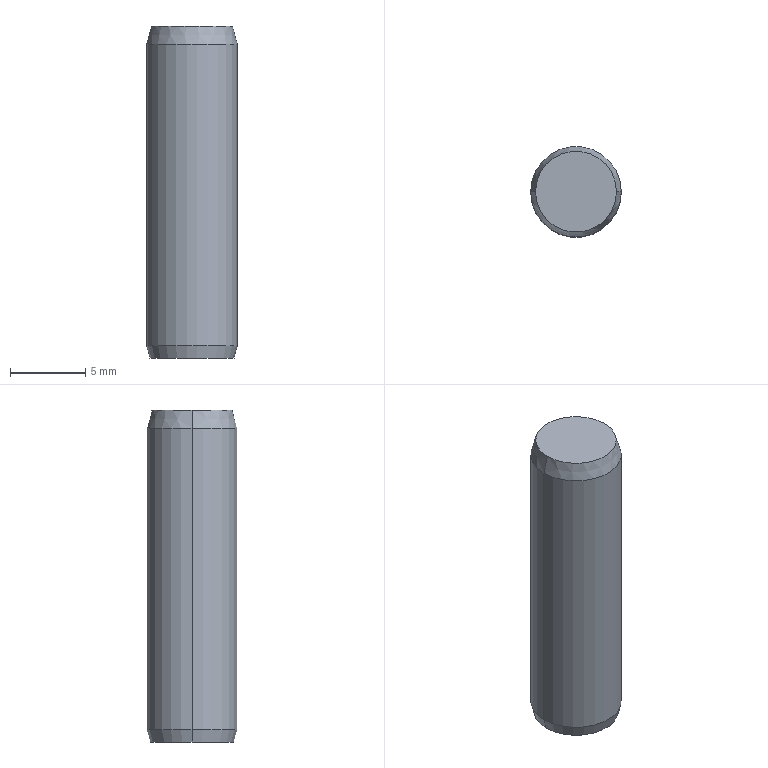Part | SolidWorks | features Chamfer 3, Cut 2, Extrusion 1, RevCut 1 | 1 solid | 16 faces | box 6 x 6 x 22 mm | volume 513.442 mm3 | cone 8 | cylinder 6 | plane 2 | commonest cylinder face diameters 3.464 x2 4.3 x2 6 x2
STEP:
#1=CARTESIAN_POINT('',(1.732,0.,1.418));
#2=VERTEX_POINT('',#1);
#3=CARTESIAN_POINT('',(-1.732,0.,1.418));
#4=VERTEX_POINT('',#3);
#5=CARTESIAN_POINT('',(0.,0.,1.418));
#6=DIRECTION('',(0.,0.,-1.));
#7=DIRECTION('',(-1.,0.,0.));
#8=AXIS2_PLACEMENT_3D('',#5,#6,#7);
#9=CIRCLE('',#8,1.732);
#10=EDGE_CURVE('',#2,#4,#9,.T.);
#11=ORIENTED_EDGE('',*,*,#10,.F.);
#12=CARTESIAN_POINT('',(2.15,0.,1.));
#13=VERTEX_POINT('',#12);
#14=CARTESIAN_POINT('',(2.15,0.,1.));
#15=DIRECTION('',(0.7071,0.,-0.7071));
#16=VECTOR('',#15,1000.);
#17=LINE('',#14,#16);
#18=EDGE_CURVE('',#2,#13,#17,.T.);
#19=ORIENTED_EDGE('',*,*,#18,.T.);
#20=CARTESIAN_POINT('',(-2.15,0.,1.));
#21=VERTEX_POINT('',#20);
#22=CARTESIAN_POINT('',(0.,0.,1.));
#23=DIRECTION('',(0.,0.,-1.));
#24=DIRECTION('',(-1.,0.,0.));
#25=AXIS2_PLACEMENT_3D('',#22,#23,#24);
#26=CIRCLE('',#25,2.15);
#27=EDGE_CURVE('',#13,#21,#26,.T.);
#28=ORIENTED_EDGE('',*,*,#27,.T.);
#29=CARTESIAN_POINT('',(-2.15,0.,1.));
#30=DIRECTION('',(-0.7071,0.,-0.7071));
#31=VECTOR('',#30,1000.);
#32=LINE('',#29,#31);
#33=EDGE_CURVE('',#4,#21,#32,.T.);
#34=ORIENTED_EDGE('',*,*,#33,.F.);
#35=EDGE_LOOP('',(#11,#19,#28,#34));
#36=FACE_OUTER_BOUND('',#35,.T.);
#37=CARTESIAN_POINT('',(0.,0.,1.));
#38=DIRECTION('',(0.,0.,-1.));
#39=DIRECTION('',(-1.,0.,0.));
#40=AXIS2_PLACEMENT_3D('',#37,#38,#39);
#41=CONICAL_SURFACE('',#40,2.15,0.7854);
#42=ADVANCED_FACE('',(#36),#41,.F.);
#43=CARTESIAN_POINT('',(-1.732,0.,10.));
#44=VERTEX_POINT('',#43);
#45=CARTESIAN_POINT('',(1.732,0.,10.));
#46=VERTEX_POINT('',#45);
#47=CARTESIAN_POINT('',(0.,0.,10.));
#48=DIRECTION('',(0.,0.,1.));
#49=DIRECTION('',(1.,0.,0.));
#50=AXIS2_PLACEMENT_3D('',#47,#48,#49);
#51=CIRCLE('',#50,1.732);
#52=EDGE_CURVE('',#44,#46,#51,.T.);
#53=ORIENTED_EDGE('',*,*,#52,.T.);
#54=CARTESIAN_POINT('',(1.732,0.,10.));
#55=DIRECTION('',(0.,0.,-1.));
#56=VECTOR('',#55,1000.);
#57=LINE('',#54,#56);
#58=EDGE_CURVE('',#46,#2,#57,.T.);
#59=ORIENTED_EDGE('',*,*,#58,.T.);
#60=ORIENTED_EDGE('',*,*,#10,.T.);
#61=CARTESIAN_POINT('',(-1.732,0.,10.));
#62=DIRECTION('',(0.,0.,-1.));
#63=VECTOR('',#62,1000.);
#64=LINE('',#61,#63);
#65=EDGE_CURVE('',#44,#4,#64,.T.);
#66=ORIENTED_EDGE('',*,*,#65,.F.);
#67=EDGE_LOOP('',(#53,#59,#60,#66));
#68=FACE_OUTER_BOUND('',#67,.T.);
#69=CARTESIAN_POINT('',(0.,0.,10.));
#70=DIRECTION('',(0.,0.,-1.));
#71=DIRECTION('',(-1.,0.,0.));
#72=AXIS2_PLACEMENT_3D('',#69,#70,#71);
#73=CYLINDRICAL_SURFACE('',#72,1.732);
#74=ADVANCED_FACE('',(#68),#73,.F.);
#75=CARTESIAN_POINT('',(0.,0.,11.));
#76=VERTEX_POINT('',#75);
#77=CARTESIAN_POINT('',(-1.732,0.,10.));
#78=DIRECTION('',(-0.866,0.,-0.5));
#79=VECTOR('',#78,1000.);
#80=LINE('',#77,#79);
#81=EDGE_CURVE('',#76,#44,#80,.T.);
#82=ORIENTED_EDGE('',*,*,#81,.F.);
#83=CARTESIAN_POINT('',(1.732,0.,10.));
#84=DIRECTION('',(0.866,0.,-0.5));
#85=VECTOR('',#84,1000.);
#86=LINE('',#83,#85);
#87=EDGE_CURVE('',#76,#46,#86,.T.);
#88=ORIENTED_EDGE('',*,*,#87,.T.);
#89=ORIENTED_EDGE('',*,*,#52,.F.);
#90=EDGE_LOOP('',(#82,#88,#89));
#91=FACE_OUTER_BOUND('',#90,.T.);
#92=CARTESIAN_POINT('',(0.,0.,10.));
#93=DIRECTION('',(0.,0.,-1.));
#94=DIRECTION('',(-1.,0.,0.));
#95=AXIS2_PLACEMENT_3D('',#92,#93,#94);
#96=CONICAL_SURFACE('',#95,1.732,1.047);
#97=ADVANCED_FACE('',(#91),#96,.F.);
#98=ORIENTED_EDGE('',*,*,#27,.F.);
#99=CARTESIAN_POINT('',(2.15,0.,0.));
#100=VERTEX_POINT('',#99);
#101=CARTESIAN_POINT('',(2.15,0.,1.));
#102=DIRECTION('',(0.,0.,-1.));
#103=VECTOR('',#102,1000.);
#104=LINE('',#101,#103);
#105=EDGE_CURVE('',#13,#100,#104,.T.);
#106=ORIENTED_EDGE('',*,*,#105,.T.);
#107=CARTESIAN_POINT('',(-2.15,0.,0.));
#108=VERTEX_POINT('',#107);
#109=CARTESIAN_POINT('',(0.,0.,0.));
#110=DIRECTION('',(0.,0.,-1.));
#111=DIRECTION('',(-1.,0.,0.));
#112=AXIS2_PLACEMENT_3D('',#109,#110,#111);
#113=CIRCLE('',#112,2.15);
#114=EDGE_CURVE('',#100,#108,#113,.T.);
#115=ORIENTED_EDGE('',*,*,#114,.T.);
#116=CARTESIAN_POINT('',(-2.15,0.,1.));
#117=DIRECTION('',(0.,0.,-1.));
#118=VECTOR('',#117,1000.);
#119=LINE('',#116,#118);
#120=EDGE_CURVE('',#21,#108,#119,.T.);
#121=ORIENTED_EDGE('',*,*,#120,.F.);
#122=EDGE_LOOP('',(#98,#106,#115,#121));
#123=FACE_OUTER_BOUND('',#122,.T.);
#124=CARTESIAN_POINT('',(0.,0.,1.));
#125=DIRECTION('',(0.,0.,-1.));
#126=DIRECTION('',(-1.,0.,0.));
#127=AXIS2_PLACEMENT_3D('',#124,#125,#126);
#128=CYLINDRICAL_SURFACE('',#127,2.15);
#129=ADVANCED_FACE('',(#123),#128,.F.);
#130=CARTESIAN_POINT('',(-2.786,0.,0.));
#131=VERTEX_POINT('',#130);
#132=CARTESIAN_POINT('',(2.786,0.,0.));
#133=VERTEX_POINT('',#132);
#134=CARTESIAN_POINT('',(0.,0.,0.));
#135=DIRECTION('',(0.,0.,-1.));
#136=DIRECTION('',(1.,0.,0.));
#137=AXIS2_PLACEMENT_3D('',#134,#135,#136);
#138=CIRCLE('',#137,2.786);
#139=EDGE_CURVE('',#131,#133,#138,.T.);
#140=ORIENTED_EDGE('',*,*,#139,.F.);
#141=CARTESIAN_POINT('',(-3.,0.,0.8));
#142=VERTEX_POINT('',#141);
#143=CARTESIAN_POINT('',(-3.,0.,0.8));
#144=DIRECTION('',(-0.2588,0.,0.9659));
#145=VECTOR('',#144,1000.);
#146=LINE('',#143,#145);
#147=EDGE_CURVE('',#131,#142,#146,.T.);
#148=ORIENTED_EDGE('',*,*,#147,.T.);
#149=CARTESIAN_POINT('',(3.,0.,0.8));
#150=VERTEX_POINT('',#149);
#151=CARTESIAN_POINT('',(0.,0.,0.8));
#152=DIRECTION('',(0.,0.,1.));
#153=DIRECTION('',(1.,0.,0.));
#154=AXIS2_PLACEMENT_3D('',#151,#152,#153);
#155=CIRCLE('',#154,3.);
#156=EDGE_CURVE('',#150,#142,#155,.T.);
#157=ORIENTED_EDGE('',*,*,#156,.F.);
#158=CARTESIAN_POINT('',(3.,0.,0.8));
#159=DIRECTION('',(0.2588,0.,0.9659));
#160=VECTOR('',#159,1000.);
#161=LINE('',#158,#160);
#162=EDGE_CURVE('',#133,#150,#161,.T.);
#163=ORIENTED_EDGE('',*,*,#162,.F.);
#164=EDGE_LOOP('',(#140,#148,#157,#163));
#165=FACE_OUTER_BOUND('',#164,.T.);
#166=CARTESIAN_POINT('',(0.,0.,0.8));
#167=DIRECTION('',(0.,0.,1.));
#168=DIRECTION('',(1.,0.,0.));
#169=AXIS2_PLACEMENT_3D('',#166,#167,#168);
#170=CONICAL_SURFACE('',#169,3.,0.2618);
#171=ADVANCED_FACE('',(#165),#170,.T.);
#172=CARTESIAN_POINT('',(2.678,0.,22.));
#173=VERTEX_POINT('',#172);
#174=CARTESIAN_POINT('',(-2.678,0.,22.));
#175=VERTEX_POINT('',#174);
#176=CARTESIAN_POINT('',(0.,0.,22.));
#177=DIRECTION('',(0.,0.,1.));
#178=DIRECTION('',(1.,0.,0.));
#179=AXIS2_PLACEMENT_3D('',#176,#177,#178);
#180=CIRCLE('',#179,2.678);
#181=EDGE_CURVE('',#173,#175,#180,.T.);
#182=ORIENTED_EDGE('',*,*,#181,.F.);
#183=CARTESIAN_POINT('',(3.,0.,20.8));
#184=VERTEX_POINT('',#183);
#185=CARTESIAN_POINT('',(2.678,0.,22.));
#186=DIRECTION('',(0.2588,0.,-0.9659));
#187=VECTOR('',#186,1000.);
#188=LINE('',#185,#187);
#189=EDGE_CURVE('',#173,#184,#188,.T.);
#190=ORIENTED_EDGE('',*,*,#189,.T.);
#191=CARTESIAN_POINT('',(-3.,0.,20.8));
#192=VERTEX_POINT('',#191);
#193=CARTESIAN_POINT('',(0.,0.,20.8));
#194=DIRECTION('',(0.,0.,-1.));
#195=DIRECTION('',(1.,0.,0.));
#196=AXIS2_PLACEMENT_3D('',#193,#194,#195);
#197=CIRCLE('',#196,3.);
#198=EDGE_CURVE('',#192,#184,#197,.T.);
#199=ORIENTED_EDGE('',*,*,#198,.F.);
#200=CARTESIAN_POINT('',(-2.678,0.,22.));
#201=DIRECTION('',(-0.2588,0.,-0.9659));
#202=VECTOR('',#201,1000.);
#203=LINE('',#200,#202);
#204=EDGE_CURVE('',#175,#192,#203,.T.);
#205=ORIENTED_EDGE('',*,*,#204,.F.);
#206=EDGE_LOOP('',(#182,#190,#199,#205));
#207=FACE_OUTER_BOUND('',#206,.T.);
#208=CARTESIAN_POINT('',(0.,0.,22.));
#209=DIRECTION('',(0.,0.,-1.));
#210=DIRECTION('',(-1.,0.,0.));
#211=AXIS2_PLACEMENT_3D('',#208,#209,#210);
#212=CONICAL_SURFACE('',#211,2.678,0.2618);
#213=ADVANCED_FACE('',(#207),#212,.T.);
#214=ORIENTED_EDGE('',*,*,#198,.T.);
#215=CARTESIAN_POINT('',(3.,0.,22.));
#216=DIRECTION('',(0.,0.,-1.));
#217=VECTOR('',#216,1000.);
#218=LINE('',#215,#217);
#219=EDGE_CURVE('',#184,#150,#218,.T.);
#220=ORIENTED_EDGE('',*,*,#219,.T.);
#221=ORIENTED_EDGE('',*,*,#156,.T.);
#222=CARTESIAN_POINT('',(-3.,0.,22.));
#223=DIRECTION('',(0.,0.,-1.));
#224=VECTOR('',#223,1000.);
#225=LINE('',#222,#224);
#226=EDGE_CURVE('',#192,#142,#225,.T.);
#227=ORIENTED_EDGE('',*,*,#226,.F.);
#228=EDGE_LOOP('',(#214,#220,#221,#227));
#229=FACE_OUTER_BOUND('',#228,.T.);
#230=CARTESIAN_POINT('',(0.,0.,22.));
#231=DIRECTION('',(0.,0.,-1.));
#232=DIRECTION('',(-1.,0.,0.));
#233=AXIS2_PLACEMENT_3D('',#230,#231,#232);
#234=CYLINDRICAL_SURFACE('',#233,3.);
#235=ADVANCED_FACE('',(#229),#234,.T.);
#236=ORIENTED_EDGE('',*,*,#219,.F.);
#237=CARTESIAN_POINT('',(0.,0.,20.8));
#238=DIRECTION('',(0.,0.,-1.));
#239=DIRECTION('',(1.,0.,0.));
#240=AXIS2_PLACEMENT_3D('',#237,#238,#239);
#241=CIRCLE('',#240,3.);
#242=EDGE_CURVE('',#184,#192,#241,.T.);
#243=ORIENTED_EDGE('',*,*,#242,.T.);
#244=ORIENTED_EDGE('',*,*,#226,.T.);
#245=CARTESIAN_POINT('',(0.,0.,0.8));
#246=DIRECTION('',(0.,0.,1.));
#247=DIRECTION('',(1.,0.,0.));
#248=AXIS2_PLACEMENT_3D('',#245,#246,#247);
#249=CIRCLE('',#248,3.);
#250=EDGE_CURVE('',#142,#150,#249,.T.);
#251=ORIENTED_EDGE('',*,*,#250,.T.);
#252=EDGE_LOOP('',(#236,#243,#244,#251));
#253=FACE_OUTER_BOUND('',#252,.T.);
#254=CARTESIAN_POINT('',(0.,0.,22.));
#255=DIRECTION('',(0.,0.,-1.));
#256=DIRECTION('',(-1.,0.,0.));
#257=AXIS2_PLACEMENT_3D('',#254,#255,#256);
#258=CYLINDRICAL_SURFACE('',#257,3.);
#259=ADVANCED_FACE('',(#253),#258,.T.);
#260=CARTESIAN_POINT('',(0.,0.,22.));
#261=DIRECTION('',(0.,0.,1.));
#262=DIRECTION('',(1.,0.,0.));
#263=AXIS2_PLACEMENT_3D('',#260,#261,#262);
#264=CIRCLE('',#263,2.678);
#265=EDGE_CURVE('',#175,#173,#264,.T.);
#266=ORIENTED_EDGE('',*,*,#265,.T.);
#267=ORIENTED_EDGE('',*,*,#181,.T.);
#268=EDGE_LOOP('',(#266,#267));
#269=FACE_OUTER_BOUND('',#268,.T.);
#270=CARTESIAN_POINT('',(0.,0.,22.));
#271=DIRECTION('',(0.,0.,1.));
#272=DIRECTION('',(1.,0.,0.));
#273=AXIS2_PLACEMENT_3D('',#270,#271,#272);
#274=PLANE('',#273);
#275=ADVANCED_FACE('',(#269),#274,.T.);
#276=CARTESIAN_POINT('',(0.,0.,0.));
#277=DIRECTION('',(0.,0.,-1.));
#278=DIRECTION('',(-1.,0.,0.));
#279=AXIS2_PLACEMENT_3D('',#276,#277,#278);
#280=CIRCLE('',#279,2.15);
#281=EDGE_CURVE('',#108,#100,#280,.T.);
#282=ORIENTED_EDGE('',*,*,#281,.F.);
#283=ORIENTED_EDGE('',*,*,#114,.F.);
#284=EDGE_LOOP('',(#282,#283));
#285=FACE_BOUND('',#284,.T.);
#286=CARTESIAN_POINT('',(0.,0.,0.));
#287=DIRECTION('',(0.,0.,-1.));
#288=DIRECTION('',(1.,0.,0.));
#289=AXIS2_PLACEMENT_3D('',#286,#287,#288);
#290=CIRCLE('',#289,2.786);
#291=EDGE_CURVE('',#133,#131,#290,.T.);
#292=ORIENTED_EDGE('',*,*,#291,.T.);
#293=ORIENTED_EDGE('',*,*,#139,.T.);
#294=EDGE_LOOP('',(#292,#293));
#295=FACE_OUTER_BOUND('',#294,.T.);
#296=CARTESIAN_POINT('',(0.,0.,0.));
#297=DIRECTION('',(0.,0.,1.));
#298=DIRECTION('',(1.,0.,0.));
#299=AXIS2_PLACEMENT_3D('',#296,#297,#298);
#300=PLANE('',#299);
#301=ADVANCED_FACE('',(#285,#295),#300,.F.);
#302=ORIENTED_EDGE('',*,*,#189,.F.);
#303=ORIENTED_EDGE('',*,*,#265,.F.);
#304=ORIENTED_EDGE('',*,*,#204,.T.);
#305=ORIENTED_EDGE('',*,*,#242,.F.);
#306=EDGE_LOOP('',(#302,#303,#304,#305));
#307=FACE_OUTER_BOUND('',#306,.T.);
#308=CARTESIAN_POINT('',(0.,0.,22.));
#309=DIRECTION('',(0.,0.,-1.));
#310=DIRECTION('',(-1.,0.,0.));
#311=AXIS2_PLACEMENT_3D('',#308,#309,#310);
#312=CONICAL_SURFACE('',#311,2.678,0.2618);
#313=ADVANCED_FACE('',(#307),#312,.T.);
#314=ORIENTED_EDGE('',*,*,#147,.F.);
#315=ORIENTED_EDGE('',*,*,#291,.F.);
#316=ORIENTED_EDGE('',*,*,#162,.T.);
#317=ORIENTED_EDGE('',*,*,#250,.F.);
#318=EDGE_LOOP('',(#314,#315,#316,#317));
#319=FACE_OUTER_BOUND('',#318,.T.);
#320=CARTESIAN_POINT('',(0.,0.,0.8));
#321=DIRECTION('',(0.,0.,1.));
#322=DIRECTION('',(1.,0.,0.));
#323=AXIS2_PLACEMENT_3D('',#320,#321,#322);
#324=CONICAL_SURFACE('',#323,3.,0.2618);
#325=ADVANCED_FACE('',(#319),#324,.T.);
#326=ORIENTED_EDGE('',*,*,#105,.F.);
#327=CARTESIAN_POINT('',(0.,0.,1.));
#328=DIRECTION('',(0.,0.,-1.));
#329=DIRECTION('',(-1.,0.,0.));
#330=AXIS2_PLACEMENT_3D('',#327,#328,#329);
#331=CIRCLE('',#330,2.15);
#332=EDGE_CURVE('',#21,#13,#331,.T.);
#333=ORIENTED_EDGE('',*,*,#332,.F.);
#334=ORIENTED_EDGE('',*,*,#120,.T.);
#335=ORIENTED_EDGE('',*,*,#281,.T.);
#336=EDGE_LOOP('',(#326,#333,#334,#335));
#337=FACE_OUTER_BOUND('',#336,.T.);
#338=CARTESIAN_POINT('',(0.,0.,1.));
#339=DIRECTION('',(0.,0.,-1.));
#340=DIRECTION('',(-1.,0.,0.));
#341=AXIS2_PLACEMENT_3D('',#338,#339,#340);
#342=CYLINDRICAL_SURFACE('',#341,2.15);
#343=ADVANCED_FACE('',(#337),#342,.F.);
#344=ORIENTED_EDGE('',*,*,#87,.F.);
#345=ORIENTED_EDGE('',*,*,#81,.T.);
#346=CARTESIAN_POINT('',(0.,0.,10.));
#347=DIRECTION('',(0.,0.,1.));
#348=DIRECTION('',(1.,0.,0.));
#349=AXIS2_PLACEMENT_3D('',#346,#347,#348);
#350=CIRCLE('',#349,1.732);
#351=EDGE_CURVE('',#46,#44,#350,.T.);
#352=ORIENTED_EDGE('',*,*,#351,.F.);
#353=EDGE_LOOP('',(#344,#345,#352));
#354=FACE_OUTER_BOUND('',#353,.T.);
#355=CARTESIAN_POINT('',(0.,0.,10.));
#356=DIRECTION('',(0.,0.,-1.));
#357=DIRECTION('',(-1.,0.,0.));
#358=AXIS2_PLACEMENT_3D('',#355,#356,#357);
#359=CONICAL_SURFACE('',#358,1.732,1.047);
#360=ADVANCED_FACE('',(#354),#359,.F.);
#361=ORIENTED_EDGE('',*,*,#58,.F.);
#362=ORIENTED_EDGE('',*,*,#351,.T.);
#363=ORIENTED_EDGE('',*,*,#65,.T.);
#364=CARTESIAN_POINT('',(0.,0.,1.418));
#365=DIRECTION('',(0.,0.,-1.));
#366=DIRECTION('',(-1.,0.,0.));
#367=AXIS2_PLACEMENT_3D('',#364,#365,#366);
#368=CIRCLE('',#367,1.732);
#369=EDGE_CURVE('',#4,#2,#368,.T.);
#370=ORIENTED_EDGE('',*,*,#369,.T.);
#371=EDGE_LOOP('',(#361,#362,#363,#370));
#372=FACE_OUTER_BOUND('',#371,.T.);
#373=CARTESIAN_POINT('',(0.,0.,10.));
#374=DIRECTION('',(0.,0.,-1.));
#375=DIRECTION('',(-1.,0.,0.));
#376=AXIS2_PLACEMENT_3D('',#373,#374,#375);
#377=CYLINDRICAL_SURFACE('',#376,1.732);
#378=ADVANCED_FACE('',(#372),#377,.F.);
#379=ORIENTED_EDGE('',*,*,#18,.F.);
#380=ORIENTED_EDGE('',*,*,#369,.F.);
#381=ORIENTED_EDGE('',*,*,#33,.T.);
#382=ORIENTED_EDGE('',*,*,#332,.T.);
#383=EDGE_LOOP('',(#379,#380,#381,#382));
#384=FACE_OUTER_BOUND('',#383,.T.);
#385=CARTESIAN_POINT('',(0.,0.,1.));
#386=DIRECTION('',(0.,0.,-1.));
#387=DIRECTION('',(-1.,0.,0.));
#388=AXIS2_PLACEMENT_3D('',#385,#386,#387);
#389=CONICAL_SURFACE('',#388,2.15,0.7854);
#390=ADVANCED_FACE('',(#384),#389,.F.);
#391=CLOSED_SHELL('',(#42,#74,#97,#129,#171,#213,#235,#259,#275,#301,#313,#325,#343,#360,#378,#390));
#392=MANIFOLD_SOLID_BREP('',#391);
#393=CARTESIAN_POINT('',(0.,0.,0.));
#394=DIRECTION('',(0.,0.,1.));
#395=DIRECTION('',(1.,0.,0.));
#396=AXIS2_PLACEMENT_3D('',#393,#394,#395);
#397=(LENGTH_UNIT()NAMED_UNIT(*)SI_UNIT(.MILLI.,.METRE.));
#398=UNCERTAINTY_MEASURE_WITH_UNIT(LENGTH_MEASURE(0.00001),#397,'','');
#399=(NAMED_UNIT(*)PLANE_ANGLE_UNIT()SI_UNIT($,.RADIAN.));
#400=(NAMED_UNIT(*)SI_UNIT($,.STERADIAN.)SOLID_ANGLE_UNIT());
#401=(GEOMETRIC_REPRESENTATION_CONTEXT(3)GLOBAL_UNCERTAINTY_ASSIGNED_CONTEXT((#398))GLOBAL_UNIT_ASSIGNED_CONTEXT((#397,#399,#400))REPRESENTATION_CONTEXT('',''));
#402=ADVANCED_BREP_SHAPE_REPRESENTATION('',(#392,#396),#401);